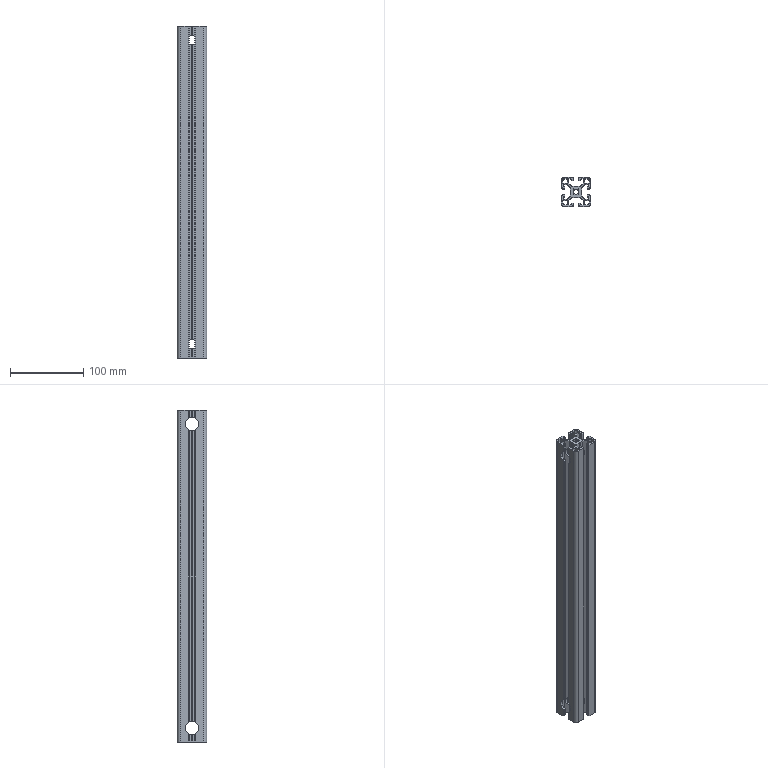Part | SolidWorks | features Extrusion 1, HoleWzd 1 | 1 solid | 273 faces | box 40 x 40 x 454 mm | volume 264516 mm3 | plane 213 | cylinder 60 | commonest cylinder face diameters 2 x16 6.8 x15 19 x12 1 x8 5 x4 9 x4